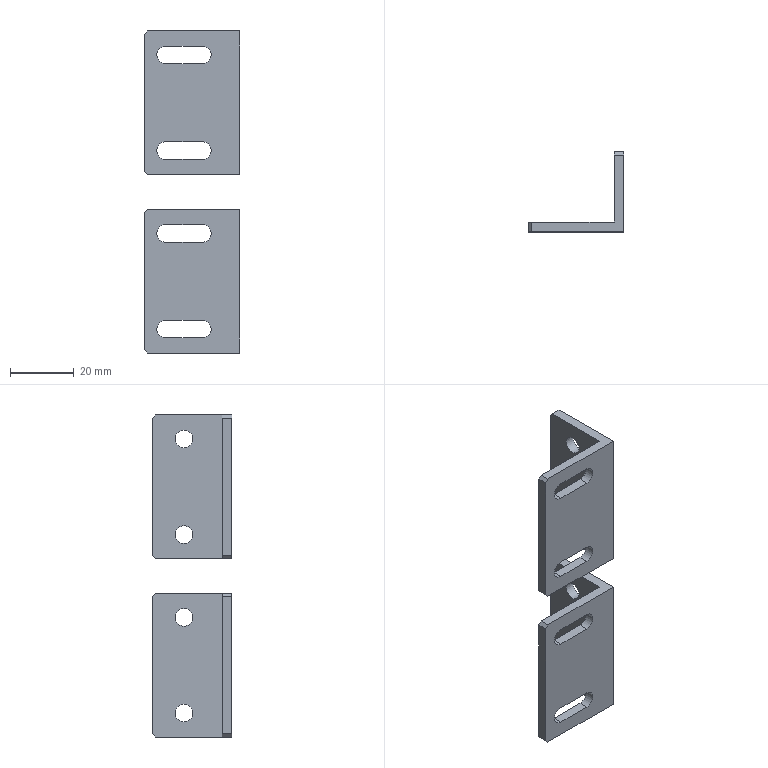Part | 2 solids | 44 faces | box 30 x 25 x 101 mm | volume 12699 mm3 | plane 32 | cylinder 12 | commonest cylinder face diameters 5.5 x12
STEP:
#1=CARTESIAN_POINT('',(-3.,25.,34.5));
#2=VERTEX_POINT('',#1);
#3=CARTESIAN_POINT('',(-3.,24.,33.5));
#4=VERTEX_POINT('',#3);
#5=CARTESIAN_POINT('',(-3.,34.5,44.));
#6=DIRECTION('',(0.,-0.7071,-0.7071));
#7=VECTOR('',#6,1000.);
#8=LINE('',#5,#7);
#9=EDGE_CURVE('',#2,#4,#8,.T.);
#10=ORIENTED_EDGE('',*,*,#9,.F.);
#11=CARTESIAN_POINT('',(0.,25.,34.5));
#12=VERTEX_POINT('',#11);
#13=CARTESIAN_POINT('',(-3.,25.,34.5));
#14=DIRECTION('',(-1.,0.,0.));
#15=VECTOR('',#14,1000.);
#16=LINE('',#13,#15);
#17=EDGE_CURVE('',#12,#2,#16,.T.);
#18=ORIENTED_EDGE('',*,*,#17,.F.);
#19=CARTESIAN_POINT('',(0.,24.,33.5));
#20=VERTEX_POINT('',#19);
#21=CARTESIAN_POINT('',(0.,24.,33.5));
#22=DIRECTION('',(0.,0.7071,0.7071));
#23=VECTOR('',#22,1000.);
#24=LINE('',#21,#23);
#25=EDGE_CURVE('',#20,#12,#24,.T.);
#26=ORIENTED_EDGE('',*,*,#25,.F.);
#27=CARTESIAN_POINT('',(0.,24.,33.5));
#28=DIRECTION('',(1.,0.,0.));
#29=VECTOR('',#28,1000.);
#30=LINE('',#27,#29);
#31=EDGE_CURVE('',#4,#20,#30,.T.);
#32=ORIENTED_EDGE('',*,*,#31,.F.);
#33=EDGE_LOOP('',(#10,#18,#26,#32));
#34=FACE_BOUND('',#33,.T.);
#35=CARTESIAN_POINT('',(0.,24.,33.5));
#36=DIRECTION('',(0.,-0.7071,0.7071));
#37=DIRECTION('',(1.,0.,0.));
#38=AXIS2_PLACEMENT_3D('',#35,#36,#37);
#39=PLANE('',#38);
#40=ADVANCED_FACE('',(#34),#39,.F.);
#41=CARTESIAN_POINT('',(-3.,24.,78.5));
#42=VERTEX_POINT('',#41);
#43=CARTESIAN_POINT('',(-3.,25.,77.5));
#44=VERTEX_POINT('',#43);
#45=CARTESIAN_POINT('',(-3.,12.,90.5));
#46=DIRECTION('',(0.,0.7071,-0.7071));
#47=VECTOR('',#46,1000.);
#48=LINE('',#45,#47);
#49=EDGE_CURVE('',#42,#44,#48,.T.);
#50=ORIENTED_EDGE('',*,*,#49,.F.);
#51=CARTESIAN_POINT('',(0.,24.,78.5));
#52=VERTEX_POINT('',#51);
#53=CARTESIAN_POINT('',(-3.,24.,78.5));
#54=DIRECTION('',(-1.,0.,0.));
#55=VECTOR('',#54,1000.);
#56=LINE('',#53,#55);
#57=EDGE_CURVE('',#52,#42,#56,.T.);
#58=ORIENTED_EDGE('',*,*,#57,.F.);
#59=CARTESIAN_POINT('',(0.,25.,77.5));
#60=VERTEX_POINT('',#59);
#61=CARTESIAN_POINT('',(0.,25.,77.5));
#62=DIRECTION('',(0.,-0.7071,0.7071));
#63=VECTOR('',#62,1000.);
#64=LINE('',#61,#63);
#65=EDGE_CURVE('',#60,#52,#64,.T.);
#66=ORIENTED_EDGE('',*,*,#65,.F.);
#67=CARTESIAN_POINT('',(0.,25.,77.5));
#68=DIRECTION('',(1.,0.,0.));
#69=VECTOR('',#68,1000.);
#70=LINE('',#67,#69);
#71=EDGE_CURVE('',#44,#60,#70,.T.);
#72=ORIENTED_EDGE('',*,*,#71,.F.);
#73=EDGE_LOOP('',(#50,#58,#66,#72));
#74=FACE_BOUND('',#73,.T.);
#75=CARTESIAN_POINT('',(-3.,25.,77.5));
#76=DIRECTION('',(0.,0.7071,0.7071));
#77=DIRECTION('',(-1.,0.,0.));
#78=AXIS2_PLACEMENT_3D('',#75,#76,#77);
#79=PLANE('',#78);
#80=ADVANCED_FACE('',(#74),#79,.T.);
#81=CARTESIAN_POINT('',(-29.,0.,78.5));
#82=VERTEX_POINT('',#81);
#83=CARTESIAN_POINT('',(-30.,0.,77.5));
#84=VERTEX_POINT('',#83);
#85=CARTESIAN_POINT('',(-30.,0.,77.5));
#86=DIRECTION('',(-0.7071,0.,-0.7071));
#87=VECTOR('',#86,1000.);
#88=LINE('',#85,#87);
#89=EDGE_CURVE('',#82,#84,#88,.T.);
#90=ORIENTED_EDGE('',*,*,#89,.F.);
#91=CARTESIAN_POINT('',(-29.,3.,78.5));
#92=VERTEX_POINT('',#91);
#93=CARTESIAN_POINT('',(-29.,0.,78.5));
#94=DIRECTION('',(0.,-1.,0.));
#95=VECTOR('',#94,1000.);
#96=LINE('',#93,#95);
#97=EDGE_CURVE('',#92,#82,#96,.T.);
#98=ORIENTED_EDGE('',*,*,#97,.F.);
#99=CARTESIAN_POINT('',(-30.,3.,77.5));
#100=VERTEX_POINT('',#99);
#101=CARTESIAN_POINT('',(-14.5,3.,93.));
#102=DIRECTION('',(0.7071,0.,0.7071));
#103=VECTOR('',#102,1000.);
#104=LINE('',#101,#103);
#105=EDGE_CURVE('',#100,#92,#104,.T.);
#106=ORIENTED_EDGE('',*,*,#105,.F.);
#107=CARTESIAN_POINT('',(-30.,3.,77.5));
#108=DIRECTION('',(0.,1.,0.));
#109=VECTOR('',#108,1000.);
#110=LINE('',#107,#109);
#111=EDGE_CURVE('',#84,#100,#110,.T.);
#112=ORIENTED_EDGE('',*,*,#111,.F.);
#113=EDGE_LOOP('',(#90,#98,#106,#112));
#114=FACE_BOUND('',#113,.T.);
#115=CARTESIAN_POINT('',(-30.,0.,77.5));
#116=DIRECTION('',(-0.7071,0.,0.7071));
#117=DIRECTION('',(0.,-1.,0.));
#118=AXIS2_PLACEMENT_3D('',#115,#116,#117);
#119=PLANE('',#118);
#120=ADVANCED_FACE('',(#114),#119,.T.);
#121=CARTESIAN_POINT('',(-30.,0.,34.5));
#122=VERTEX_POINT('',#121);
#123=CARTESIAN_POINT('',(-29.,0.,33.5));
#124=VERTEX_POINT('',#123);
#125=CARTESIAN_POINT('',(-29.,0.,33.5));
#126=DIRECTION('',(0.7071,0.,-0.7071));
#127=VECTOR('',#126,1000.);
#128=LINE('',#125,#127);
#129=EDGE_CURVE('',#122,#124,#128,.T.);
#130=ORIENTED_EDGE('',*,*,#129,.F.);
#131=CARTESIAN_POINT('',(-30.,3.,34.5));
#132=VERTEX_POINT('',#131);
#133=CARTESIAN_POINT('',(-30.,0.,34.5));
#134=DIRECTION('',(0.,-1.,0.));
#135=VECTOR('',#134,1000.);
#136=LINE('',#133,#135);
#137=EDGE_CURVE('',#132,#122,#136,.T.);
#138=ORIENTED_EDGE('',*,*,#137,.F.);
#139=CARTESIAN_POINT('',(-29.,3.,33.5));
#140=VERTEX_POINT('',#139);
#141=CARTESIAN_POINT('',(-37.,3.,41.5));
#142=DIRECTION('',(-0.7071,0.,0.7071));
#143=VECTOR('',#142,1000.);
#144=LINE('',#141,#143);
#145=EDGE_CURVE('',#140,#132,#144,.T.);
#146=ORIENTED_EDGE('',*,*,#145,.F.);
#147=CARTESIAN_POINT('',(-29.,0.,33.5));
#148=DIRECTION('',(0.,1.,0.));
#149=VECTOR('',#148,1000.);
#150=LINE('',#147,#149);
#151=EDGE_CURVE('',#124,#140,#150,.T.);
#152=ORIENTED_EDGE('',*,*,#151,.F.);
#153=EDGE_LOOP('',(#130,#138,#146,#152));
#154=FACE_BOUND('',#153,.T.);
#155=CARTESIAN_POINT('',(-29.,0.,33.5));
#156=DIRECTION('',(0.7071,0.,0.7071));
#157=DIRECTION('',(0.,1.,0.));
#158=AXIS2_PLACEMENT_3D('',#155,#156,#157);
#159=PLANE('',#158);
#160=ADVANCED_FACE('',(#154),#159,.F.);
#161=CARTESIAN_POINT('',(-11.75,3.,43.75));
#162=VERTEX_POINT('',#161);
#163=CARTESIAN_POINT('',(-11.75,0.,43.75));
#164=VERTEX_POINT('',#163);
#165=CARTESIAN_POINT('',(-11.75,3.,43.75));
#166=DIRECTION('',(0.,-1.,0.));
#167=VECTOR('',#166,1000.);
#168=LINE('',#165,#167);
#169=EDGE_CURVE('',#162,#164,#168,.T.);
#170=ORIENTED_EDGE('',*,*,#169,.T.);
#171=CARTESIAN_POINT('',(-23.25,0.,43.75));
#172=VERTEX_POINT('',#171);
#173=CARTESIAN_POINT('',(-23.25,0.,43.75));
#174=DIRECTION('',(1.,0.,0.));
#175=VECTOR('',#174,1000.);
#176=LINE('',#173,#175);
#177=EDGE_CURVE('',#172,#164,#176,.T.);
#178=ORIENTED_EDGE('',*,*,#177,.F.);
#179=CARTESIAN_POINT('',(-23.25,3.,43.75));
#180=VERTEX_POINT('',#179);
#181=CARTESIAN_POINT('',(-23.25,3.,43.75));
#182=DIRECTION('',(0.,1.,0.));
#183=VECTOR('',#182,1000.);
#184=LINE('',#181,#183);
#185=EDGE_CURVE('',#172,#180,#184,.T.);
#186=ORIENTED_EDGE('',*,*,#185,.T.);
#187=CARTESIAN_POINT('',(-23.25,3.,43.75));
#188=DIRECTION('',(1.,0.,0.));
#189=VECTOR('',#188,1000.);
#190=LINE('',#187,#189);
#191=EDGE_CURVE('',#180,#162,#190,.T.);
#192=ORIENTED_EDGE('',*,*,#191,.T.);
#193=EDGE_LOOP('',(#170,#178,#186,#192));
#194=FACE_BOUND('',#193,.T.);
#195=CARTESIAN_POINT('',(-23.25,3.,43.75));
#196=DIRECTION('',(0.,0.,1.));
#197=DIRECTION('',(1.,0.,0.));
#198=AXIS2_PLACEMENT_3D('',#195,#196,#197);
#199=PLANE('',#198);
#200=ADVANCED_FACE('',(#194),#199,.F.);
#201=CARTESIAN_POINT('',(-11.75,0.,38.25));
#202=VERTEX_POINT('',#201);
#203=CARTESIAN_POINT('',(-11.75,3.,38.25));
#204=VERTEX_POINT('',#203);
#205=CARTESIAN_POINT('',(-11.75,3.,38.25));
#206=DIRECTION('',(0.,1.,0.));
#207=VECTOR('',#206,1000.);
#208=LINE('',#205,#207);
#209=EDGE_CURVE('',#202,#204,#208,.T.);
#210=ORIENTED_EDGE('',*,*,#209,.T.);
#211=CARTESIAN_POINT('',(-23.25,3.,38.25));
#212=VERTEX_POINT('',#211);
#213=CARTESIAN_POINT('',(-23.25,3.,38.25));
#214=DIRECTION('',(1.,0.,0.));
#215=VECTOR('',#214,1000.);
#216=LINE('',#213,#215);
#217=EDGE_CURVE('',#212,#204,#216,.T.);
#218=ORIENTED_EDGE('',*,*,#217,.F.);
#219=CARTESIAN_POINT('',(-23.25,0.,38.25));
#220=VERTEX_POINT('',#219);
#221=CARTESIAN_POINT('',(-23.25,3.,38.25));
#222=DIRECTION('',(0.,-1.,0.));
#223=VECTOR('',#222,1000.);
#224=LINE('',#221,#223);
#225=EDGE_CURVE('',#212,#220,#224,.T.);
#226=ORIENTED_EDGE('',*,*,#225,.T.);
#227=CARTESIAN_POINT('',(-23.25,0.,38.25));
#228=DIRECTION('',(1.,0.,0.));
#229=VECTOR('',#228,1000.);
#230=LINE('',#227,#229);
#231=EDGE_CURVE('',#220,#202,#230,.T.);
#232=ORIENTED_EDGE('',*,*,#231,.T.);
#233=EDGE_LOOP('',(#210,#218,#226,#232));
#234=FACE_BOUND('',#233,.T.);
#235=CARTESIAN_POINT('',(-23.25,3.,38.25));
#236=DIRECTION('',(0.,0.,-1.));
#237=DIRECTION('',(-1.,0.,0.));
#238=AXIS2_PLACEMENT_3D('',#235,#236,#237);
#239=PLANE('',#238);
#240=ADVANCED_FACE('',(#234),#239,.F.);
#241=CARTESIAN_POINT('',(-23.25,3.,41.));
#242=DIRECTION('',(0.,1.,0.));
#243=DIRECTION('',(0.,0.,1.));
#244=AXIS2_PLACEMENT_3D('',#241,#242,#243);
#245=CIRCLE('',#244,2.75);
#246=EDGE_CURVE('',#212,#180,#245,.T.);
#247=ORIENTED_EDGE('',*,*,#246,.T.);
#248=ORIENTED_EDGE('',*,*,#185,.F.);
#249=CARTESIAN_POINT('',(-23.25,0.,41.));
#250=DIRECTION('',(0.,1.,0.));
#251=DIRECTION('',(0.,0.,1.));
#252=AXIS2_PLACEMENT_3D('',#249,#250,#251);
#253=CIRCLE('',#252,2.75);
#254=EDGE_CURVE('',#220,#172,#253,.T.);
#255=ORIENTED_EDGE('',*,*,#254,.F.);
#256=ORIENTED_EDGE('',*,*,#225,.F.);
#257=EDGE_LOOP('',(#247,#248,#255,#256));
#258=FACE_BOUND('',#257,.T.);
#259=CARTESIAN_POINT('',(-23.25,3.,41.));
#260=DIRECTION('',(0.,1.,0.));
#261=DIRECTION('',(0.,0.,1.));
#262=AXIS2_PLACEMENT_3D('',#259,#260,#261);
#263=CYLINDRICAL_SURFACE('',#262,2.75);
#264=ADVANCED_FACE('',(#258),#263,.F.);
#265=CARTESIAN_POINT('',(-11.75,0.,41.));
#266=DIRECTION('',(0.,1.,0.));
#267=DIRECTION('',(0.,0.,1.));
#268=AXIS2_PLACEMENT_3D('',#265,#266,#267);
#269=CIRCLE('',#268,2.75);
#270=EDGE_CURVE('',#164,#202,#269,.T.);
#271=ORIENTED_EDGE('',*,*,#270,.F.);
#272=ORIENTED_EDGE('',*,*,#169,.F.);
#273=CARTESIAN_POINT('',(-11.75,3.,41.));
#274=DIRECTION('',(0.,1.,0.));
#275=DIRECTION('',(0.,0.,1.));
#276=AXIS2_PLACEMENT_3D('',#273,#274,#275);
#277=CIRCLE('',#276,2.75);
#278=EDGE_CURVE('',#162,#204,#277,.T.);
#279=ORIENTED_EDGE('',*,*,#278,.T.);
#280=ORIENTED_EDGE('',*,*,#209,.F.);
#281=EDGE_LOOP('',(#271,#272,#279,#280));
#282=FACE_BOUND('',#281,.T.);
#283=CARTESIAN_POINT('',(-11.75,3.,41.));
#284=DIRECTION('',(0.,1.,0.));
#285=DIRECTION('',(0.,0.,1.));
#286=AXIS2_PLACEMENT_3D('',#283,#284,#285);
#287=CYLINDRICAL_SURFACE('',#286,2.75);
#288=ADVANCED_FACE('',(#282),#287,.F.);
#289=CARTESIAN_POINT('',(-11.75,3.,73.75));
#290=VERTEX_POINT('',#289);
#291=CARTESIAN_POINT('',(-11.75,0.,73.75));
#292=VERTEX_POINT('',#291);
#293=CARTESIAN_POINT('',(-11.75,3.,73.75));
#294=DIRECTION('',(0.,-1.,0.));
#295=VECTOR('',#294,1000.);
#296=LINE('',#293,#295);
#297=EDGE_CURVE('',#290,#292,#296,.T.);
#298=ORIENTED_EDGE('',*,*,#297,.T.);
#299=CARTESIAN_POINT('',(-23.25,0.,73.75));
#300=VERTEX_POINT('',#299);
#301=CARTESIAN_POINT('',(-23.25,0.,73.75));
#302=DIRECTION('',(1.,0.,0.));
#303=VECTOR('',#302,1000.);
#304=LINE('',#301,#303);
#305=EDGE_CURVE('',#300,#292,#304,.T.);
#306=ORIENTED_EDGE('',*,*,#305,.F.);
#307=CARTESIAN_POINT('',(-23.25,3.,73.75));
#308=VERTEX_POINT('',#307);
#309=CARTESIAN_POINT('',(-23.25,3.,73.75));
#310=DIRECTION('',(0.,1.,0.));
#311=VECTOR('',#310,1000.);
#312=LINE('',#309,#311);
#313=EDGE_CURVE('',#300,#308,#312,.T.);
#314=ORIENTED_EDGE('',*,*,#313,.T.);
#315=CARTESIAN_POINT('',(-23.25,3.,73.75));
#316=DIRECTION('',(1.,0.,0.));
#317=VECTOR('',#316,1000.);
#318=LINE('',#315,#317);
#319=EDGE_CURVE('',#308,#290,#318,.T.);
#320=ORIENTED_EDGE('',*,*,#319,.T.);
#321=EDGE_LOOP('',(#298,#306,#314,#320));
#322=FACE_BOUND('',#321,.T.);
#323=CARTESIAN_POINT('',(-23.25,3.,73.75));
#324=DIRECTION('',(0.,0.,1.));
#325=DIRECTION('',(1.,0.,0.));
#326=AXIS2_PLACEMENT_3D('',#323,#324,#325);
#327=PLANE('',#326);
#328=ADVANCED_FACE('',(#322),#327,.F.);
#329=CARTESIAN_POINT('',(-11.75,0.,68.25));
#330=VERTEX_POINT('',#329);
#331=CARTESIAN_POINT('',(-11.75,3.,68.25));
#332=VERTEX_POINT('',#331);
#333=CARTESIAN_POINT('',(-11.75,3.,68.25));
#334=DIRECTION('',(0.,1.,0.));
#335=VECTOR('',#334,1000.);
#336=LINE('',#333,#335);
#337=EDGE_CURVE('',#330,#332,#336,.T.);
#338=ORIENTED_EDGE('',*,*,#337,.T.);
#339=CARTESIAN_POINT('',(-23.25,3.,68.25));
#340=VERTEX_POINT('',#339);
#341=CARTESIAN_POINT('',(-23.25,3.,68.25));
#342=DIRECTION('',(1.,0.,0.));
#343=VECTOR('',#342,1000.);
#344=LINE('',#341,#343);
#345=EDGE_CURVE('',#340,#332,#344,.T.);
#346=ORIENTED_EDGE('',*,*,#345,.F.);
#347=CARTESIAN_POINT('',(-23.25,0.,68.25));
#348=VERTEX_POINT('',#347);
#349=CARTESIAN_POINT('',(-23.25,3.,68.25));
#350=DIRECTION('',(0.,-1.,0.));
#351=VECTOR('',#350,1000.);
#352=LINE('',#349,#351);
#353=EDGE_CURVE('',#340,#348,#352,.T.);
#354=ORIENTED_EDGE('',*,*,#353,.T.);
#355=CARTESIAN_POINT('',(-23.25,0.,68.25));
#356=DIRECTION('',(1.,0.,0.));
#357=VECTOR('',#356,1000.);
#358=LINE('',#355,#357);
#359=EDGE_CURVE('',#348,#330,#358,.T.);
#360=ORIENTED_EDGE('',*,*,#359,.T.);
#361=EDGE_LOOP('',(#338,#346,#354,#360));
#362=FACE_BOUND('',#361,.T.);
#363=CARTESIAN_POINT('',(-23.25,3.,68.25));
#364=DIRECTION('',(0.,0.,-1.));
#365=DIRECTION('',(-1.,0.,0.));
#366=AXIS2_PLACEMENT_3D('',#363,#364,#365);
#367=PLANE('',#366);
#368=ADVANCED_FACE('',(#362),#367,.F.);
#369=CARTESIAN_POINT('',(-23.25,3.,71.));
#370=DIRECTION('',(0.,1.,0.));
#371=DIRECTION('',(0.,0.,1.));
#372=AXIS2_PLACEMENT_3D('',#369,#370,#371);
#373=CIRCLE('',#372,2.75);
#374=EDGE_CURVE('',#340,#308,#373,.T.);
#375=ORIENTED_EDGE('',*,*,#374,.T.);
#376=ORIENTED_EDGE('',*,*,#313,.F.);
#377=CARTESIAN_POINT('',(-23.25,0.,71.));
#378=DIRECTION('',(0.,1.,0.));
#379=DIRECTION('',(0.,0.,1.));
#380=AXIS2_PLACEMENT_3D('',#377,#378,#379);
#381=CIRCLE('',#380,2.75);
#382=EDGE_CURVE('',#348,#300,#381,.T.);
#383=ORIENTED_EDGE('',*,*,#382,.F.);
#384=ORIENTED_EDGE('',*,*,#353,.F.);
#385=EDGE_LOOP('',(#375,#376,#383,#384));
#386=FACE_BOUND('',#385,.T.);
#387=CARTESIAN_POINT('',(-23.25,3.,71.));
#388=DIRECTION('',(0.,1.,0.));
#389=DIRECTION('',(0.,0.,1.));
#390=AXIS2_PLACEMENT_3D('',#387,#388,#389);
#391=CYLINDRICAL_SURFACE('',#390,2.75);
#392=ADVANCED_FACE('',(#386),#391,.F.);
#393=CARTESIAN_POINT('',(-11.75,0.,71.));
#394=DIRECTION('',(0.,1.,0.));
#395=DIRECTION('',(0.,0.,1.));
#396=AXIS2_PLACEMENT_3D('',#393,#394,#395);
#397=CIRCLE('',#396,2.75);
#398=EDGE_CURVE('',#292,#330,#397,.T.);
#399=ORIENTED_EDGE('',*,*,#398,.F.);
#400=ORIENTED_EDGE('',*,*,#297,.F.);
#401=CARTESIAN_POINT('',(-11.75,3.,71.));
#402=DIRECTION('',(0.,1.,0.));
#403=DIRECTION('',(0.,0.,1.));
#404=AXIS2_PLACEMENT_3D('',#401,#402,#403);
#405=CIRCLE('',#404,2.75);
#406=EDGE_CURVE('',#290,#332,#405,.T.);
#407=ORIENTED_EDGE('',*,*,#406,.T.);
#408=ORIENTED_EDGE('',*,*,#337,.F.);
#409=EDGE_LOOP('',(#399,#400,#407,#408));
#410=FACE_BOUND('',#409,.T.);
#411=CARTESIAN_POINT('',(-11.75,3.,71.));
#412=DIRECTION('',(0.,1.,0.));
#413=DIRECTION('',(0.,0.,1.));
#414=AXIS2_PLACEMENT_3D('',#411,#412,#413);
#415=CYLINDRICAL_SURFACE('',#414,2.75);
#416=ADVANCED_FACE('',(#410),#415,.F.);
#417=CARTESIAN_POINT('',(-3.,15.,43.75));
#418=VERTEX_POINT('',#417);
#419=CARTESIAN_POINT('',(-3.,15.,41.));
#420=DIRECTION('',(-1.,0.,0.));
#421=DIRECTION('',(0.,0.,1.));
#422=AXIS2_PLACEMENT_3D('',#419,#420,#421);
#423=CIRCLE('',#422,2.75);
#424=EDGE_CURVE('',#418,#418,#423,.T.);
#425=ORIENTED_EDGE('',*,*,#424,.T.);
#426=EDGE_LOOP('',(#425));
#427=FACE_BOUND('',#426,.T.);
#428=CARTESIAN_POINT('',(0.,15.,43.75));
#429=VERTEX_POINT('',#428);
#430=CARTESIAN_POINT('',(0.,15.,41.));
#431=DIRECTION('',(-1.,0.,0.));
#432=DIRECTION('',(0.,0.,1.));
#433=AXIS2_PLACEMENT_3D('',#430,#431,#432);
#434=CIRCLE('',#433,2.75);
#435=EDGE_CURVE('',#429,#429,#434,.T.);
#436=ORIENTED_EDGE('',*,*,#435,.F.);
#437=EDGE_LOOP('',(#436));
#438=FACE_BOUND('',#437,.T.);
#439=CARTESIAN_POINT('',(-3.,15.,41.));
#440=DIRECTION('',(-1.,0.,0.));
#441=DIRECTION('',(0.,0.,1.));
#442=AXIS2_PLACEMENT_3D('',#439,#440,#441);
#443=CYLINDRICAL_SURFACE('',#442,2.75);
#444=ADVANCED_FACE('',(#427,#438),#443,.F.);
#445=CARTESIAN_POINT('',(-3.,15.,73.75));
#446=VERTEX_POINT('',#445);
#447=CARTESIAN_POINT('',(-3.,15.,71.));
#448=DIRECTION('',(-1.,0.,0.));
#449=DIRECTION('',(0.,0.,1.));
#450=AXIS2_PLACEMENT_3D('',#447,#448,#449);
#451=CIRCLE('',#450,2.75);
#452=EDGE_CURVE('',#446,#446,#451,.T.);
#453=ORIENTED_EDGE('',*,*,#452,.T.);
#454=EDGE_LOOP('',(#453));
#455=FACE_BOUND('',#454,.T.);
#456=CARTESIAN_POINT('',(0.,15.,73.75));
#457=VERTEX_POINT('',#456);
#458=CARTESIAN_POINT('',(0.,15.,71.));
#459=DIRECTION('',(-1.,0.,0.));
#460=DIRECTION('',(0.,0.,1.));
#461=AXIS2_PLACEMENT_3D('',#458,#459,#460);
#462=CIRCLE('',#461,2.75);
#463=EDGE_CURVE('',#457,#457,#462,.T.);
#464=ORIENTED_EDGE('',*,*,#463,.F.);
#465=EDGE_LOOP('',(#464));
#466=FACE_BOUND('',#465,.T.);
#467=CARTESIAN_POINT('',(-3.,15.,71.));
#468=DIRECTION('',(-1.,0.,0.));
#469=DIRECTION('',(0.,0.,1.));
#470=AXIS2_PLACEMENT_3D('',#467,#468,#469);
#471=CYLINDRICAL_SURFACE('',#470,2.75);
#472=ADVANCED_FACE('',(#455,#466),#471,.F.);
#473=CARTESIAN_POINT('',(0.,0.,33.5));
#474=VERTEX_POINT('',#473);
#475=CARTESIAN_POINT('',(0.,0.,33.5));
#476=DIRECTION('',(1.,0.,0.));
#477=VECTOR('',#476,1000.);
#478=LINE('',#475,#477);
#479=EDGE_CURVE('',#124,#474,#478,.T.);
#480=ORIENTED_EDGE('',*,*,#479,.F.);
#481=ORIENTED_EDGE('',*,*,#151,.T.);
#482=CARTESIAN_POINT('',(-3.,3.,33.5));
#483=VERTEX_POINT('',#482);
#484=CARTESIAN_POINT('',(0.,3.,33.5));
#485=DIRECTION('',(1.,0.,0.));
#486=VECTOR('',#485,1000.);
#487=LINE('',#484,#486);
#488=EDGE_CURVE('',#140,#483,#487,.T.);
#489=ORIENTED_EDGE('',*,*,#488,.T.);
#490=CARTESIAN_POINT('',(-3.,0.,33.5));
#491=DIRECTION('',(0.,1.,0.));
#492=VECTOR('',#491,1000.);
#493=LINE('',#490,#492);
#494=EDGE_CURVE('',#483,#4,#493,.T.);
#495=ORIENTED_EDGE('',*,*,#494,.T.);
#496=ORIENTED_EDGE('',*,*,#31,.T.);
#497=CARTESIAN_POINT('',(0.,0.,33.5));
#498=DIRECTION('',(0.,1.,0.));
#499=VECTOR('',#498,1000.);
#500=LINE('',#497,#499);
#501=EDGE_CURVE('',#474,#20,#500,.T.);
#502=ORIENTED_EDGE('',*,*,#501,.F.);
#503=EDGE_LOOP('',(#480,#481,#489,#495,#496,#502));
#504=FACE_BOUND('',#503,.T.);
#505=CARTESIAN_POINT('',(0.,0.,33.5));
#506=DIRECTION('',(0.,0.,-1.));
#507=DIRECTION('',(-1.,0.,0.));
#508=AXIS2_PLACEMENT_3D('',#505,#506,#507);
#509=PLANE('',#508);
#510=ADVANCED_FACE('',(#504),#509,.T.);
#511=CARTESIAN_POINT('',(-3.,3.,78.5));
#512=VERTEX_POINT('',#511);
#513=CARTESIAN_POINT('',(0.,3.,78.5));
#514=DIRECTION('',(1.,0.,0.));
#515=VECTOR('',#514,1000.);
#516=LINE('',#513,#515);
#517=EDGE_CURVE('',#92,#512,#516,.T.);
#518=ORIENTED_EDGE('',*,*,#517,.F.);
#519=ORIENTED_EDGE('',*,*,#97,.T.);
#520=CARTESIAN_POINT('',(0.,0.,78.5));
#521=VERTEX_POINT('',#520);
#522=CARTESIAN_POINT('',(0.,0.,78.5));
#523=DIRECTION('',(1.,0.,0.));
#524=VECTOR('',#523,1000.);
#525=LINE('',#522,#524);
#526=EDGE_CURVE('',#82,#521,#525,.T.);
#527=ORIENTED_EDGE('',*,*,#526,.T.);
#528=CARTESIAN_POINT('',(0.,0.,78.5));
#529=DIRECTION('',(0.,1.,0.));
#530=VECTOR('',#529,1000.);
#531=LINE('',#528,#530);
#532=EDGE_CURVE('',#521,#52,#531,.T.);
#533=ORIENTED_EDGE('',*,*,#532,.T.);
#534=ORIENTED_EDGE('',*,*,#57,.T.);
#535=CARTESIAN_POINT('',(-3.,0.,78.5));
#536=DIRECTION('',(0.,1.,0.));
#537=VECTOR('',#536,1000.);
#538=LINE('',#535,#537);
#539=EDGE_CURVE('',#512,#42,#538,.T.);
#540=ORIENTED_EDGE('',*,*,#539,.F.);
#541=EDGE_LOOP('',(#518,#519,#527,#533,#534,#540));
#542=FACE_BOUND('',#541,.T.);
#543=CARTESIAN_POINT('',(0.,0.,78.5));
#544=DIRECTION('',(0.,0.,-1.));
#545=DIRECTION('',(-1.,0.,0.));
#546=AXIS2_PLACEMENT_3D('',#543,#544,#545);
#547=PLANE('',#546);
#548=ADVANCED_FACE('',(#542),#547,.F.);
#549=CARTESIAN_POINT('',(-30.,0.,78.5));
#550=DIRECTION('',(0.,0.,-1.));
#551=VECTOR('',#550,1000.);
#552=LINE('',#549,#551);
#553=EDGE_CURVE('',#84,#122,#552,.T.);
#554=ORIENTED_EDGE('',*,*,#553,.T.);
#555=ORIENTED_EDGE('',*,*,#129,.T.);
#556=ORIENTED_EDGE('',*,*,#479,.T.);
#557=CARTESIAN_POINT('',(0.,0.,78.5));
#558=DIRECTION('',(0.,0.,-1.));
#559=VECTOR('',#558,1000.);
#560=LINE('',#557,#559);
#561=EDGE_CURVE('',#521,#474,#560,.T.);
#562=ORIENTED_EDGE('',*,*,#561,.F.);
#563=ORIENTED_EDGE('',*,*,#526,.F.);
#564=ORIENTED_EDGE('',*,*,#89,.T.);
#565=EDGE_LOOP('',(#554,#555,#556,#562,#563,#564));
#566=FACE_BOUND('',#565,.T.);
#567=ORIENTED_EDGE('',*,*,#305,.T.);
#568=ORIENTED_EDGE('',*,*,#398,.T.);
#569=ORIENTED_EDGE('',*,*,#359,.F.);
#570=ORIENTED_EDGE('',*,*,#382,.T.);
#571=EDGE_LOOP('',(#567,#568,#569,#570));
#572=FACE_BOUND('',#571,.T.);
#573=ORIENTED_EDGE('',*,*,#254,.T.);
#574=ORIENTED_EDGE('',*,*,#177,.T.);
#575=ORIENTED_EDGE('',*,*,#270,.T.);
#576=ORIENTED_EDGE('',*,*,#231,.F.);
#577=EDGE_LOOP('',(#573,#574,#575,#576));
#578=FACE_BOUND('',#577,.T.);
#579=CARTESIAN_POINT('',(0.,0.,78.5));
#580=DIRECTION('',(0.,1.,0.));
#581=DIRECTION('',(-1.,0.,0.));
#582=AXIS2_PLACEMENT_3D('',#579,#580,#581);
#583=PLANE('',#582);
#584=ADVANCED_FACE('',(#566,#572,#578),#583,.F.);
#585=CARTESIAN_POINT('',(-30.,3.,78.5));
#586=DIRECTION('',(0.,0.,-1.));
#587=VECTOR('',#586,1000.);
#588=LINE('',#585,#587);
#589=EDGE_CURVE('',#100,#132,#588,.T.);
#590=ORIENTED_EDGE('',*,*,#589,.T.);
#591=ORIENTED_EDGE('',*,*,#137,.T.);
#592=ORIENTED_EDGE('',*,*,#553,.F.);
#593=ORIENTED_EDGE('',*,*,#111,.T.);
#594=EDGE_LOOP('',(#590,#591,#592,#593));
#595=FACE_BOUND('',#594,.T.);
#596=CARTESIAN_POINT('',(-30.,0.,78.5));
#597=DIRECTION('',(-1.,0.,0.));
#598=DIRECTION('',(0.,0.,1.));
#599=AXIS2_PLACEMENT_3D('',#596,#597,#598);
#600=PLANE('',#599);
#601=ADVANCED_FACE('',(#595),#600,.T.);
#602=ORIENTED_EDGE('',*,*,#488,.F.);
#603=ORIENTED_EDGE('',*,*,#145,.T.);
#604=ORIENTED_EDGE('',*,*,#589,.F.);
#605=ORIENTED_EDGE('',*,*,#105,.T.);
#606=ORIENTED_EDGE('',*,*,#517,.T.);
#607=CARTESIAN_POINT('',(-3.,3.,78.5));
#608=DIRECTION('',(0.,0.,-1.));
#609=VECTOR('',#608,1000.);
#610=LINE('',#607,#609);
#611=EDGE_CURVE('',#512,#483,#610,.T.);
#612=ORIENTED_EDGE('',*,*,#611,.T.);
#613=EDGE_LOOP('',(#602,#603,#604,#605,#606,#612));
#614=FACE_BOUND('',#613,.T.);
#615=ORIENTED_EDGE('',*,*,#319,.F.);
#616=ORIENTED_EDGE('',*,*,#374,.F.);
#617=ORIENTED_EDGE('',*,*,#345,.T.);
#618=ORIENTED_EDGE('',*,*,#406,.F.);
#619=EDGE_LOOP('',(#615,#616,#617,#618));
#620=FACE_BOUND('',#619,.T.);
#621=ORIENTED_EDGE('',*,*,#246,.F.);
#622=ORIENTED_EDGE('',*,*,#217,.T.);
#623=ORIENTED_EDGE('',*,*,#278,.F.);
#624=ORIENTED_EDGE('',*,*,#191,.F.);
#625=EDGE_LOOP('',(#621,#622,#623,#624));
#626=FACE_BOUND('',#625,.T.);
#627=CARTESIAN_POINT('',(0.,3.,78.5));
#628=DIRECTION('',(0.,1.,0.));
#629=DIRECTION('',(-1.,0.,0.));
#630=AXIS2_PLACEMENT_3D('',#627,#628,#629);
#631=PLANE('',#630);
#632=ADVANCED_FACE('',(#614,#620,#626),#631,.T.);
#633=ORIENTED_EDGE('',*,*,#539,.T.);
#634=ORIENTED_EDGE('',*,*,#49,.T.);
#635=CARTESIAN_POINT('',(-3.,25.,78.5));
#636=DIRECTION('',(0.,0.,-1.));
#637=VECTOR('',#636,1000.);
#638=LINE('',#635,#637);
#639=EDGE_CURVE('',#44,#2,#638,.T.);
#640=ORIENTED_EDGE('',*,*,#639,.T.);
#641=ORIENTED_EDGE('',*,*,#9,.T.);
#642=ORIENTED_EDGE('',*,*,#494,.F.);
#643=ORIENTED_EDGE('',*,*,#611,.F.);
#644=EDGE_LOOP('',(#633,#634,#640,#641,#642,#643));
#645=FACE_BOUND('',#644,.T.);
#646=ORIENTED_EDGE('',*,*,#452,.F.);
#647=EDGE_LOOP('',(#646));
#648=FACE_BOUND('',#647,.T.);
#649=ORIENTED_EDGE('',*,*,#424,.F.);
#650=EDGE_LOOP('',(#649));
#651=FACE_BOUND('',#650,.T.);
#652=CARTESIAN_POINT('',(-3.,0.,78.5));
#653=DIRECTION('',(-1.,0.,0.));
#654=DIRECTION('',(0.,0.,1.));
#655=AXIS2_PLACEMENT_3D('',#652,#653,#654);
#656=PLANE('',#655);
#657=ADVANCED_FACE('',(#645,#648,#651),#656,.T.);
#658=ORIENTED_EDGE('',*,*,#639,.F.);
#659=ORIENTED_EDGE('',*,*,#71,.T.);
#660=CARTESIAN_POINT('',(0.,25.,78.5));
#661=DIRECTION('',(0.,0.,-1.));
#662=VECTOR('',#661,1000.);
#663=LINE('',#660,#662);
#664=EDGE_CURVE('',#60,#12,#663,.T.);
#665=ORIENTED_EDGE('',*,*,#664,.T.);
#666=ORIENTED_EDGE('',*,*,#17,.T.);
#667=EDGE_LOOP('',(#658,#659,#665,#666));
#668=FACE_BOUND('',#667,.T.);
#669=CARTESIAN_POINT('',(-3.,25.,78.5));
#670=DIRECTION('',(0.,1.,0.));
#671=DIRECTION('',(0.,0.,1.));
#672=AXIS2_PLACEMENT_3D('',#669,#670,#671);
#673=PLANE('',#672);
#674=ADVANCED_FACE('',(#668),#673,.T.);
#675=ORIENTED_EDGE('',*,*,#664,.F.);
#676=ORIENTED_EDGE('',*,*,#65,.T.);
#677=ORIENTED_EDGE('',*,*,#532,.F.);
#678=ORIENTED_EDGE('',*,*,#561,.T.);
#679=ORIENTED_EDGE('',*,*,#501,.T.);
#680=ORIENTED_EDGE('',*,*,#25,.T.);
#681=EDGE_LOOP('',(#675,#676,#677,#678,#679,#680));
#682=FACE_BOUND('',#681,.T.);
#683=ORIENTED_EDGE('',*,*,#463,.T.);
#684=EDGE_LOOP('',(#683));
#685=FACE_BOUND('',#684,.T.);
#686=ORIENTED_EDGE('',*,*,#435,.T.);
#687=EDGE_LOOP('',(#686));
#688=FACE_BOUND('',#687,.T.);
#689=CARTESIAN_POINT('',(0.,0.,78.5));
#690=DIRECTION('',(-1.,0.,0.));
#691=DIRECTION('',(0.,0.,1.));
#692=AXIS2_PLACEMENT_3D('',#689,#690,#691);
#693=PLANE('',#692);
#694=ADVANCED_FACE('',(#682,#685,#688),#693,.F.);
#695=CLOSED_SHELL('',(#40,#80,#120,#160,#200,#240,#264,#288,#328,#368,#392,#416,#444,#472,#510,#548,#584,#601,#632,#657,#674,#694));
#696=MANIFOLD_SOLID_BREP('',#695);
#697=CARTESIAN_POINT('',(-3.,25.,-21.5));
#698=VERTEX_POINT('',#697);
#699=CARTESIAN_POINT('',(-3.,24.,-22.5));
#700=VERTEX_POINT('',#699);
#701=CARTESIAN_POINT('',(-3.,34.5,-12.));
#702=DIRECTION('',(0.,-0.7071,-0.7071));
#703=VECTOR('',#702,1000.);
#704=LINE('',#701,#703);
#705=EDGE_CURVE('',#698,#700,#704,.T.);
#706=ORIENTED_EDGE('',*,*,#705,.F.);
#707=CARTESIAN_POINT('',(0.,25.,-21.5));
#708=VERTEX_POINT('',#707);
#709=CARTESIAN_POINT('',(-3.,25.,-21.5));
#710=DIRECTION('',(-1.,0.,0.));
#711=VECTOR('',#710,1000.);
#712=LINE('',#709,#711);
#713=EDGE_CURVE('',#708,#698,#712,.T.);
#714=ORIENTED_EDGE('',*,*,#713,.F.);
#715=CARTESIAN_POINT('',(0.,24.,-22.5));
#716=VERTEX_POINT('',#715);
#717=CARTESIAN_POINT('',(0.,24.,-22.5));
#718=DIRECTION('',(0.,0.7071,0.7071));
#719=VECTOR('',#718,1000.);
#720=LINE('',#717,#719);
#721=EDGE_CURVE('',#716,#708,#720,.T.);
#722=ORIENTED_EDGE('',*,*,#721,.F.);
#723=CARTESIAN_POINT('',(0.,24.,-22.5));
#724=DIRECTION('',(1.,0.,0.));
#725=VECTOR('',#724,1000.);
#726=LINE('',#723,#725);
#727=EDGE_CURVE('',#700,#716,#726,.T.);
#728=ORIENTED_EDGE('',*,*,#727,.F.);
#729=EDGE_LOOP('',(#706,#714,#722,#728));
#730=FACE_BOUND('',#729,.T.);
#731=CARTESIAN_POINT('',(0.,24.,-22.5));
#732=DIRECTION('',(0.,-0.7071,0.7071));
#733=DIRECTION('',(1.,0.,0.));
#734=AXIS2_PLACEMENT_3D('',#731,#732,#733);
#735=PLANE('',#734);
#736=ADVANCED_FACE('',(#730),#735,.F.);
#737=CARTESIAN_POINT('',(-3.,24.,22.5));
#738=VERTEX_POINT('',#737);
#739=CARTESIAN_POINT('',(-3.,25.,21.5));
#740=VERTEX_POINT('',#739);
#741=CARTESIAN_POINT('',(-3.,12.,34.5));
#742=DIRECTION('',(0.,0.7071,-0.7071));
#743=VECTOR('',#742,1000.);
#744=LINE('',#741,#743);
#745=EDGE_CURVE('',#738,#740,#744,.T.);
#746=ORIENTED_EDGE('',*,*,#745,.F.);
#747=CARTESIAN_POINT('',(0.,24.,22.5));
#748=VERTEX_POINT('',#747);
#749=CARTESIAN_POINT('',(-3.,24.,22.5));
#750=DIRECTION('',(-1.,0.,0.));
#751=VECTOR('',#750,1000.);
#752=LINE('',#749,#751);
#753=EDGE_CURVE('',#748,#738,#752,.T.);
#754=ORIENTED_EDGE('',*,*,#753,.F.);
#755=CARTESIAN_POINT('',(0.,25.,21.5));
#756=VERTEX_POINT('',#755);
#757=CARTESIAN_POINT('',(0.,25.,21.5));
#758=DIRECTION('',(0.,-0.7071,0.7071));
#759=VECTOR('',#758,1000.);
#760=LINE('',#757,#759);
#761=EDGE_CURVE('',#756,#748,#760,.T.);
#762=ORIENTED_EDGE('',*,*,#761,.F.);
#763=CARTESIAN_POINT('',(0.,25.,21.5));
#764=DIRECTION('',(1.,0.,0.));
#765=VECTOR('',#764,1000.);
#766=LINE('',#763,#765);
#767=EDGE_CURVE('',#740,#756,#766,.T.);
#768=ORIENTED_EDGE('',*,*,#767,.F.);
#769=EDGE_LOOP('',(#746,#754,#762,#768));
#770=FACE_BOUND('',#769,.T.);
#771=CARTESIAN_POINT('',(-3.,25.,21.5));
#772=DIRECTION('',(0.,0.7071,0.7071));
#773=DIRECTION('',(-1.,0.,0.));
#774=AXIS2_PLACEMENT_3D('',#771,#772,#773);
#775=PLANE('',#774);
#776=ADVANCED_FACE('',(#770),#775,.T.);
#777=CARTESIAN_POINT('',(-29.,0.,22.5));
#778=VERTEX_POINT('',#777);
#779=CARTESIAN_POINT('',(-30.,0.,21.5));
#780=VERTEX_POINT('',#779);
#781=CARTESIAN_POINT('',(-30.,0.,21.5));
#782=DIRECTION('',(-0.7071,0.,-0.7071));
#783=VECTOR('',#782,1000.);
#784=LINE('',#781,#783);
#785=EDGE_CURVE('',#778,#780,#784,.T.);
#786=ORIENTED_EDGE('',*,*,#785,.F.);
#787=CARTESIAN_POINT('',(-29.,3.,22.5));
#788=VERTEX_POINT('',#787);
#789=CARTESIAN_POINT('',(-29.,0.,22.5));
#790=DIRECTION('',(0.,-1.,0.));
#791=VECTOR('',#790,1000.);
#792=LINE('',#789,#791);
#793=EDGE_CURVE('',#788,#778,#792,.T.);
#794=ORIENTED_EDGE('',*,*,#793,.F.);
#795=CARTESIAN_POINT('',(-30.,3.,21.5));
#796=VERTEX_POINT('',#795);
#797=CARTESIAN_POINT('',(-14.5,3.,37.));
#798=DIRECTION('',(0.7071,0.,0.7071));
#799=VECTOR('',#798,1000.);
#800=LINE('',#797,#799);
#801=EDGE_CURVE('',#796,#788,#800,.T.);
#802=ORIENTED_EDGE('',*,*,#801,.F.);
#803=CARTESIAN_POINT('',(-30.,3.,21.5));
#804=DIRECTION('',(0.,1.,0.));
#805=VECTOR('',#804,1000.);
#806=LINE('',#803,#805);
#807=EDGE_CURVE('',#780,#796,#806,.T.);
#808=ORIENTED_EDGE('',*,*,#807,.F.);
#809=EDGE_LOOP('',(#786,#794,#802,#808));
#810=FACE_BOUND('',#809,.T.);
#811=CARTESIAN_POINT('',(-30.,0.,21.5));
#812=DIRECTION('',(-0.7071,0.,0.7071));
#813=DIRECTION('',(0.,-1.,0.));
#814=AXIS2_PLACEMENT_3D('',#811,#812,#813);
#815=PLANE('',#814);
#816=ADVANCED_FACE('',(#810),#815,.T.);
#817=CARTESIAN_POINT('',(-30.,0.,-21.5));
#818=VERTEX_POINT('',#817);
#819=CARTESIAN_POINT('',(-29.,0.,-22.5));
#820=VERTEX_POINT('',#819);
#821=CARTESIAN_POINT('',(-29.,0.,-22.5));
#822=DIRECTION('',(0.7071,0.,-0.7071));
#823=VECTOR('',#822,1000.);
#824=LINE('',#821,#823);
#825=EDGE_CURVE('',#818,#820,#824,.T.);
#826=ORIENTED_EDGE('',*,*,#825,.F.);
#827=CARTESIAN_POINT('',(-30.,3.,-21.5));
#828=VERTEX_POINT('',#827);
#829=CARTESIAN_POINT('',(-30.,0.,-21.5));
#830=DIRECTION('',(0.,-1.,0.));
#831=VECTOR('',#830,1000.);
#832=LINE('',#829,#831);
#833=EDGE_CURVE('',#828,#818,#832,.T.);
#834=ORIENTED_EDGE('',*,*,#833,.F.);
#835=CARTESIAN_POINT('',(-29.,3.,-22.5));
#836=VERTEX_POINT('',#835);
#837=CARTESIAN_POINT('',(-37.,3.,-14.5));
#838=DIRECTION('',(-0.7071,0.,0.7071));
#839=VECTOR('',#838,1000.);
#840=LINE('',#837,#839);
#841=EDGE_CURVE('',#836,#828,#840,.T.);
#842=ORIENTED_EDGE('',*,*,#841,.F.);
#843=CARTESIAN_POINT('',(-29.,0.,-22.5));
#844=DIRECTION('',(0.,1.,0.));
#845=VECTOR('',#844,1000.);
#846=LINE('',#843,#845);
#847=EDGE_CURVE('',#820,#836,#846,.T.);
#848=ORIENTED_EDGE('',*,*,#847,.F.);
#849=EDGE_LOOP('',(#826,#834,#842,#848));
#850=FACE_BOUND('',#849,.T.);
#851=CARTESIAN_POINT('',(-29.,0.,-22.5));
#852=DIRECTION('',(0.7071,0.,0.7071));
#853=DIRECTION('',(0.,1.,0.));
#854=AXIS2_PLACEMENT_3D('',#851,#852,#853);
#855=PLANE('',#854);
#856=ADVANCED_FACE('',(#850),#855,.F.);
#857=CARTESIAN_POINT('',(-11.75,3.,-12.25));
#858=VERTEX_POINT('',#857);
#859=CARTESIAN_POINT('',(-11.75,0.,-12.25));
#860=VERTEX_POINT('',#859);
#861=CARTESIAN_POINT('',(-11.75,3.,-12.25));
#862=DIRECTION('',(0.,-1.,0.));
#863=VECTOR('',#862,1000.);
#864=LINE('',#861,#863);
#865=EDGE_CURVE('',#858,#860,#864,.T.);
#866=ORIENTED_EDGE('',*,*,#865,.T.);
#867=CARTESIAN_POINT('',(-23.25,0.,-12.25));
#868=VERTEX_POINT('',#867);
#869=CARTESIAN_POINT('',(-23.25,0.,-12.25));
#870=DIRECTION('',(1.,0.,0.));
#871=VECTOR('',#870,1000.);
#872=LINE('',#869,#871);
#873=EDGE_CURVE('',#868,#860,#872,.T.);
#874=ORIENTED_EDGE('',*,*,#873,.F.);
#875=CARTESIAN_POINT('',(-23.25,3.,-12.25));
#876=VERTEX_POINT('',#875);
#877=CARTESIAN_POINT('',(-23.25,3.,-12.25));
#878=DIRECTION('',(0.,1.,0.));
#879=VECTOR('',#878,1000.);
#880=LINE('',#877,#879);
#881=EDGE_CURVE('',#868,#876,#880,.T.);
#882=ORIENTED_EDGE('',*,*,#881,.T.);
#883=CARTESIAN_POINT('',(-23.25,3.,-12.25));
#884=DIRECTION('',(1.,0.,0.));
#885=VECTOR('',#884,1000.);
#886=LINE('',#883,#885);
#887=EDGE_CURVE('',#876,#858,#886,.T.);
#888=ORIENTED_EDGE('',*,*,#887,.T.);
#889=EDGE_LOOP('',(#866,#874,#882,#888));
#890=FACE_BOUND('',#889,.T.);
#891=CARTESIAN_POINT('',(-23.25,3.,-12.25));
#892=DIRECTION('',(0.,0.,1.));
#893=DIRECTION('',(1.,0.,0.));
#894=AXIS2_PLACEMENT_3D('',#891,#892,#893);
#895=PLANE('',#894);
#896=ADVANCED_FACE('',(#890),#895,.F.);
#897=CARTESIAN_POINT('',(-11.75,0.,-17.75));
#898=VERTEX_POINT('',#897);
#899=CARTESIAN_POINT('',(-11.75,3.,-17.75));
#900=VERTEX_POINT('',#899);
#901=CARTESIAN_POINT('',(-11.75,3.,-17.75));
#902=DIRECTION('',(0.,1.,0.));
#903=VECTOR('',#902,1000.);
#904=LINE('',#901,#903);
#905=EDGE_CURVE('',#898,#900,#904,.T.);
#906=ORIENTED_EDGE('',*,*,#905,.T.);
#907=CARTESIAN_POINT('',(-23.25,3.,-17.75));
#908=VERTEX_POINT('',#907);
#909=CARTESIAN_POINT('',(-23.25,3.,-17.75));
#910=DIRECTION('',(1.,0.,0.));
#911=VECTOR('',#910,1000.);
#912=LINE('',#909,#911);
#913=EDGE_CURVE('',#908,#900,#912,.T.);
#914=ORIENTED_EDGE('',*,*,#913,.F.);
#915=CARTESIAN_POINT('',(-23.25,0.,-17.75));
#916=VERTEX_POINT('',#915);
#917=CARTESIAN_POINT('',(-23.25,3.,-17.75));
#918=DIRECTION('',(0.,-1.,0.));
#919=VECTOR('',#918,1000.);
#920=LINE('',#917,#919);
#921=EDGE_CURVE('',#908,#916,#920,.T.);
#922=ORIENTED_EDGE('',*,*,#921,.T.);
#923=CARTESIAN_POINT('',(-23.25,0.,-17.75));
#924=DIRECTION('',(1.,0.,0.));
#925=VECTOR('',#924,1000.);
#926=LINE('',#923,#925);
#927=EDGE_CURVE('',#916,#898,#926,.T.);
#928=ORIENTED_EDGE('',*,*,#927,.T.);
#929=EDGE_LOOP('',(#906,#914,#922,#928));
#930=FACE_BOUND('',#929,.T.);
#931=CARTESIAN_POINT('',(-23.25,3.,-17.75));
#932=DIRECTION('',(0.,0.,-1.));
#933=DIRECTION('',(-1.,0.,0.));
#934=AXIS2_PLACEMENT_3D('',#931,#932,#933);
#935=PLANE('',#934);
#936=ADVANCED_FACE('',(#930),#935,.F.);
#937=CARTESIAN_POINT('',(-23.25,3.,-15.));
#938=DIRECTION('',(0.,1.,0.));
#939=DIRECTION('',(0.,0.,1.));
#940=AXIS2_PLACEMENT_3D('',#937,#938,#939);
#941=CIRCLE('',#940,2.75);
#942=EDGE_CURVE('',#908,#876,#941,.T.);
#943=ORIENTED_EDGE('',*,*,#942,.T.);
#944=ORIENTED_EDGE('',*,*,#881,.F.);
#945=CARTESIAN_POINT('',(-23.25,0.,-15.));
#946=DIRECTION('',(0.,1.,0.));
#947=DIRECTION('',(0.,0.,1.));
#948=AXIS2_PLACEMENT_3D('',#945,#946,#947);
#949=CIRCLE('',#948,2.75);
#950=EDGE_CURVE('',#916,#868,#949,.T.);
#951=ORIENTED_EDGE('',*,*,#950,.F.);
#952=ORIENTED_EDGE('',*,*,#921,.F.);
#953=EDGE_LOOP('',(#943,#944,#951,#952));
#954=FACE_BOUND('',#953,.T.);
#955=CARTESIAN_POINT('',(-23.25,3.,-15.));
#956=DIRECTION('',(0.,1.,0.));
#957=DIRECTION('',(0.,0.,1.));
#958=AXIS2_PLACEMENT_3D('',#955,#956,#957);
#959=CYLINDRICAL_SURFACE('',#958,2.75);
#960=ADVANCED_FACE('',(#954),#959,.F.);
#961=CARTESIAN_POINT('',(-11.75,0.,-15.));
#962=DIRECTION('',(0.,1.,0.));
#963=DIRECTION('',(0.,0.,1.));
#964=AXIS2_PLACEMENT_3D('',#961,#962,#963);
#965=CIRCLE('',#964,2.75);
#966=EDGE_CURVE('',#860,#898,#965,.T.);
#967=ORIENTED_EDGE('',*,*,#966,.F.);
#968=ORIENTED_EDGE('',*,*,#865,.F.);
#969=CARTESIAN_POINT('',(-11.75,3.,-15.));
#970=DIRECTION('',(0.,1.,0.));
#971=DIRECTION('',(0.,0.,1.));
#972=AXIS2_PLACEMENT_3D('',#969,#970,#971);
#973=CIRCLE('',#972,2.75);
#974=EDGE_CURVE('',#858,#900,#973,.T.);
#975=ORIENTED_EDGE('',*,*,#974,.T.);
#976=ORIENTED_EDGE('',*,*,#905,.F.);
#977=EDGE_LOOP('',(#967,#968,#975,#976));
#978=FACE_BOUND('',#977,.T.);
#979=CARTESIAN_POINT('',(-11.75,3.,-15.));
#980=DIRECTION('',(0.,1.,0.));
#981=DIRECTION('',(0.,0.,1.));
#982=AXIS2_PLACEMENT_3D('',#979,#980,#981);
#983=CYLINDRICAL_SURFACE('',#982,2.75);
#984=ADVANCED_FACE('',(#978),#983,.F.);
#985=CARTESIAN_POINT('',(-11.75,3.,17.75));
#986=VERTEX_POINT('',#985);
#987=CARTESIAN_POINT('',(-11.75,0.,17.75));
#988=VERTEX_POINT('',#987);
#989=CARTESIAN_POINT('',(-11.75,3.,17.75));
#990=DIRECTION('',(0.,-1.,0.));
#991=VECTOR('',#990,1000.);
#992=LINE('',#989,#991);
#993=EDGE_CURVE('',#986,#988,#992,.T.);
#994=ORIENTED_EDGE('',*,*,#993,.T.);
#995=CARTESIAN_POINT('',(-23.25,0.,17.75));
#996=VERTEX_POINT('',#995);
#997=CARTESIAN_POINT('',(-23.25,0.,17.75));
#998=DIRECTION('',(1.,0.,0.));
#999=VECTOR('',#998,1000.);
#1000=LINE('',#997,#999);
#1001=EDGE_CURVE('',#996,#988,#1000,.T.);
#1002=ORIENTED_EDGE('',*,*,#1001,.F.);
#1003=CARTESIAN_POINT('',(-23.25,3.,17.75));
#1004=VERTEX_POINT('',#1003);
#1005=CARTESIAN_POINT('',(-23.25,3.,17.75));
#1006=DIRECTION('',(0.,1.,0.));
#1007=VECTOR('',#1006,1000.);
#1008=LINE('',#1005,#1007);
#1009=EDGE_CURVE('',#996,#1004,#1008,.T.);
#1010=ORIENTED_EDGE('',*,*,#1009,.T.);
#1011=CARTESIAN_POINT('',(-23.25,3.,17.75));
#1012=DIRECTION('',(1.,0.,0.));
#1013=VECTOR('',#1012,1000.);
#1014=LINE('',#1011,#1013);
#1015=EDGE_CURVE('',#1004,#986,#1014,.T.);
#1016=ORIENTED_EDGE('',*,*,#1015,.T.);
#1017=EDGE_LOOP('',(#994,#1002,#1010,#1016));
#1018=FACE_BOUND('',#1017,.T.);
#1019=CARTESIAN_POINT('',(-23.25,3.,17.75));
#1020=DIRECTION('',(0.,0.,1.));
#1021=DIRECTION('',(1.,0.,0.));
#1022=AXIS2_PLACEMENT_3D('',#1019,#1020,#1021);
#1023=PLANE('',#1022);
#1024=ADVANCED_FACE('',(#1018),#1023,.F.);
#1025=CARTESIAN_POINT('',(-11.75,0.,12.25));
#1026=VERTEX_POINT('',#1025);
#1027=CARTESIAN_POINT('',(-11.75,3.,12.25));
#1028=VERTEX_POINT('',#1027);
#1029=CARTESIAN_POINT('',(-11.75,3.,12.25));
#1030=DIRECTION('',(0.,1.,0.));
#1031=VECTOR('',#1030,1000.);
#1032=LINE('',#1029,#1031);
#1033=EDGE_CURVE('',#1026,#1028,#1032,.T.);
#1034=ORIENTED_EDGE('',*,*,#1033,.T.);
#1035=CARTESIAN_POINT('',(-23.25,3.,12.25));
#1036=VERTEX_POINT('',#1035);
#1037=CARTESIAN_POINT('',(-23.25,3.,12.25));
#1038=DIRECTION('',(1.,0.,0.));
#1039=VECTOR('',#1038,1000.);
#1040=LINE('',#1037,#1039);
#1041=EDGE_CURVE('',#1036,#1028,#1040,.T.);
#1042=ORIENTED_EDGE('',*,*,#1041,.F.);
#1043=CARTESIAN_POINT('',(-23.25,0.,12.25));
#1044=VERTEX_POINT('',#1043);
#1045=CARTESIAN_POINT('',(-23.25,3.,12.25));
#1046=DIRECTION('',(0.,-1.,0.));
#1047=VECTOR('',#1046,1000.);
#1048=LINE('',#1045,#1047);
#1049=EDGE_CURVE('',#1036,#1044,#1048,.T.);
#1050=ORIENTED_EDGE('',*,*,#1049,.T.);
#1051=CARTESIAN_POINT('',(-23.25,0.,12.25));
#1052=DIRECTION('',(1.,0.,0.));
#1053=VECTOR('',#1052,1000.);
#1054=LINE('',#1051,#1053);
#1055=EDGE_CURVE('',#1044,#1026,#1054,.T.);
#1056=ORIENTED_EDGE('',*,*,#1055,.T.);
#1057=EDGE_LOOP('',(#1034,#1042,#1050,#1056));
#1058=FACE_BOUND('',#1057,.T.);
#1059=CARTESIAN_POINT('',(-23.25,3.,12.25));
#1060=DIRECTION('',(0.,0.,-1.));
#1061=DIRECTION('',(-1.,0.,0.));
#1062=AXIS2_PLACEMENT_3D('',#1059,#1060,#1061);
#1063=PLANE('',#1062);
#1064=ADVANCED_FACE('',(#1058),#1063,.F.);
#1065=CARTESIAN_POINT('',(-23.25,3.,15.));
#1066=DIRECTION('',(0.,1.,0.));
#1067=DIRECTION('',(0.,0.,1.));
#1068=AXIS2_PLACEMENT_3D('',#1065,#1066,#1067);
#1069=CIRCLE('',#1068,2.75);
#1070=EDGE_CURVE('',#1036,#1004,#1069,.T.);
#1071=ORIENTED_EDGE('',*,*,#1070,.T.);
#1072=ORIENTED_EDGE('',*,*,#1009,.F.);
#1073=CARTESIAN_POINT('',(-23.25,0.,15.));
#1074=DIRECTION('',(0.,1.,0.));
#1075=DIRECTION('',(0.,0.,1.));
#1076=AXIS2_PLACEMENT_3D('',#1073,#1074,#1075);
#1077=CIRCLE('',#1076,2.75);
#1078=EDGE_CURVE('',#1044,#996,#1077,.T.);
#1079=ORIENTED_EDGE('',*,*,#1078,.F.);
#1080=ORIENTED_EDGE('',*,*,#1049,.F.);
#1081=EDGE_LOOP('',(#1071,#1072,#1079,#1080));
#1082=FACE_BOUND('',#1081,.T.);
#1083=CARTESIAN_POINT('',(-23.25,3.,15.));
#1084=DIRECTION('',(0.,1.,0.));
#1085=DIRECTION('',(0.,0.,1.));
#1086=AXIS2_PLACEMENT_3D('',#1083,#1084,#1085);
#1087=CYLINDRICAL_SURFACE('',#1086,2.75);
#1088=ADVANCED_FACE('',(#1082),#1087,.F.);
#1089=CARTESIAN_POINT('',(-11.75,0.,15.));
#1090=DIRECTION('',(0.,1.,0.));
#1091=DIRECTION('',(0.,0.,1.));
#1092=AXIS2_PLACEMENT_3D('',#1089,#1090,#1091);
#1093=CIRCLE('',#1092,2.75);
#1094=EDGE_CURVE('',#988,#1026,#1093,.T.);
#1095=ORIENTED_EDGE('',*,*,#1094,.F.);
#1096=ORIENTED_EDGE('',*,*,#993,.F.);
#1097=CARTESIAN_POINT('',(-11.75,3.,15.));
#1098=DIRECTION('',(0.,1.,0.));
#1099=DIRECTION('',(0.,0.,1.));
#1100=AXIS2_PLACEMENT_3D('',#1097,#1098,#1099);
#1101=CIRCLE('',#1100,2.75);
#1102=EDGE_CURVE('',#986,#1028,#1101,.T.);
#1103=ORIENTED_EDGE('',*,*,#1102,.T.);
#1104=ORIENTED_EDGE('',*,*,#1033,.F.);
#1105=EDGE_LOOP('',(#1095,#1096,#1103,#1104));
#1106=FACE_BOUND('',#1105,.T.);
#1107=CARTESIAN_POINT('',(-11.75,3.,15.));
#1108=DIRECTION('',(0.,1.,0.));
#1109=DIRECTION('',(0.,0.,1.));
#1110=AXIS2_PLACEMENT_3D('',#1107,#1108,#1109);
#1111=CYLINDRICAL_SURFACE('',#1110,2.75);
#1112=ADVANCED_FACE('',(#1106),#1111,.F.);
#1113=CARTESIAN_POINT('',(-3.,15.,-12.25));
#1114=VERTEX_POINT('',#1113);
#1115=CARTESIAN_POINT('',(-3.,15.,-15.));
#1116=DIRECTION('',(-1.,0.,0.));
#1117=DIRECTION('',(0.,0.,1.));
#1118=AXIS2_PLACEMENT_3D('',#1115,#1116,#1117);
#1119=CIRCLE('',#1118,2.75);
#1120=EDGE_CURVE('',#1114,#1114,#1119,.T.);
#1121=ORIENTED_EDGE('',*,*,#1120,.T.);
#1122=EDGE_LOOP('',(#1121));
#1123=FACE_BOUND('',#1122,.T.);
#1124=CARTESIAN_POINT('',(0.,15.,-12.25));
#1125=VERTEX_POINT('',#1124);
#1126=CARTESIAN_POINT('',(0.,15.,-15.));
#1127=DIRECTION('',(-1.,0.,0.));
#1128=DIRECTION('',(0.,0.,1.));
#1129=AXIS2_PLACEMENT_3D('',#1126,#1127,#1128);
#1130=CIRCLE('',#1129,2.75);
#1131=EDGE_CURVE('',#1125,#1125,#1130,.T.);
#1132=ORIENTED_EDGE('',*,*,#1131,.F.);
#1133=EDGE_LOOP('',(#1132));
#1134=FACE_BOUND('',#1133,.T.);
#1135=CARTESIAN_POINT('',(-3.,15.,-15.));
#1136=DIRECTION('',(-1.,0.,0.));
#1137=DIRECTION('',(0.,0.,1.));
#1138=AXIS2_PLACEMENT_3D('',#1135,#1136,#1137);
#1139=CYLINDRICAL_SURFACE('',#1138,2.75);
#1140=ADVANCED_FACE('',(#1123,#1134),#1139,.F.);
#1141=CARTESIAN_POINT('',(-3.,15.,17.75));
#1142=VERTEX_POINT('',#1141);
#1143=CARTESIAN_POINT('',(-3.,15.,15.));
#1144=DIRECTION('',(-1.,0.,0.));
#1145=DIRECTION('',(0.,0.,1.));
#1146=AXIS2_PLACEMENT_3D('',#1143,#1144,#1145);
#1147=CIRCLE('',#1146,2.75);
#1148=EDGE_CURVE('',#1142,#1142,#1147,.T.);
#1149=ORIENTED_EDGE('',*,*,#1148,.T.);
#1150=EDGE_LOOP('',(#1149));
#1151=FACE_BOUND('',#1150,.T.);
#1152=CARTESIAN_POINT('',(0.,15.,17.75));
#1153=VERTEX_POINT('',#1152);
#1154=CARTESIAN_POINT('',(0.,15.,15.));
#1155=DIRECTION('',(-1.,0.,0.));
#1156=DIRECTION('',(0.,0.,1.));
#1157=AXIS2_PLACEMENT_3D('',#1154,#1155,#1156);
#1158=CIRCLE('',#1157,2.75);
#1159=EDGE_CURVE('',#1153,#1153,#1158,.T.);
#1160=ORIENTED_EDGE('',*,*,#1159,.F.);
#1161=EDGE_LOOP('',(#1160));
#1162=FACE_BOUND('',#1161,.T.);
#1163=CARTESIAN_POINT('',(-3.,15.,15.));
#1164=DIRECTION('',(-1.,0.,0.));
#1165=DIRECTION('',(0.,0.,1.));
#1166=AXIS2_PLACEMENT_3D('',#1163,#1164,#1165);
#1167=CYLINDRICAL_SURFACE('',#1166,2.75);
#1168=ADVANCED_FACE('',(#1151,#1162),#1167,.F.);
#1169=CARTESIAN_POINT('',(0.,0.,-22.5));
#1170=VERTEX_POINT('',#1169);
#1171=CARTESIAN_POINT('',(0.,0.,-22.5));
#1172=DIRECTION('',(1.,0.,0.));
#1173=VECTOR('',#1172,1000.);
#1174=LINE('',#1171,#1173);
#1175=EDGE_CURVE('',#820,#1170,#1174,.T.);
#1176=ORIENTED_EDGE('',*,*,#1175,.F.);
#1177=ORIENTED_EDGE('',*,*,#847,.T.);
#1178=CARTESIAN_POINT('',(-3.,3.,-22.5));
#1179=VERTEX_POINT('',#1178);
#1180=CARTESIAN_POINT('',(0.,3.,-22.5));
#1181=DIRECTION('',(1.,0.,0.));
#1182=VECTOR('',#1181,1000.);
#1183=LINE('',#1180,#1182);
#1184=EDGE_CURVE('',#836,#1179,#1183,.T.);
#1185=ORIENTED_EDGE('',*,*,#1184,.T.);
#1186=CARTESIAN_POINT('',(-3.,0.,-22.5));
#1187=DIRECTION('',(0.,1.,0.));
#1188=VECTOR('',#1187,1000.);
#1189=LINE('',#1186,#1188);
#1190=EDGE_CURVE('',#1179,#700,#1189,.T.);
#1191=ORIENTED_EDGE('',*,*,#1190,.T.);
#1192=ORIENTED_EDGE('',*,*,#727,.T.);
#1193=CARTESIAN_POINT('',(0.,0.,-22.5));
#1194=DIRECTION('',(0.,1.,0.));
#1195=VECTOR('',#1194,1000.);
#1196=LINE('',#1193,#1195);
#1197=EDGE_CURVE('',#1170,#716,#1196,.T.);
#1198=ORIENTED_EDGE('',*,*,#1197,.F.);
#1199=EDGE_LOOP('',(#1176,#1177,#1185,#1191,#1192,#1198));
#1200=FACE_BOUND('',#1199,.T.);
#1201=CARTESIAN_POINT('',(0.,0.,-22.5));
#1202=DIRECTION('',(0.,0.,-1.));
#1203=DIRECTION('',(-1.,0.,0.));
#1204=AXIS2_PLACEMENT_3D('',#1201,#1202,#1203);
#1205=PLANE('',#1204);
#1206=ADVANCED_FACE('',(#1200),#1205,.T.);
#1207=CARTESIAN_POINT('',(-3.,3.,22.5));
#1208=VERTEX_POINT('',#1207);
#1209=CARTESIAN_POINT('',(0.,3.,22.5));
#1210=DIRECTION('',(1.,0.,0.));
#1211=VECTOR('',#1210,1000.);
#1212=LINE('',#1209,#1211);
#1213=EDGE_CURVE('',#788,#1208,#1212,.T.);
#1214=ORIENTED_EDGE('',*,*,#1213,.F.);
#1215=ORIENTED_EDGE('',*,*,#793,.T.);
#1216=CARTESIAN_POINT('',(0.,0.,22.5));
#1217=VERTEX_POINT('',#1216);
#1218=CARTESIAN_POINT('',(0.,0.,22.5));
#1219=DIRECTION('',(1.,0.,0.));
#1220=VECTOR('',#1219,1000.);
#1221=LINE('',#1218,#1220);
#1222=EDGE_CURVE('',#778,#1217,#1221,.T.);
#1223=ORIENTED_EDGE('',*,*,#1222,.T.);
#1224=CARTESIAN_POINT('',(0.,0.,22.5));
#1225=DIRECTION('',(0.,1.,0.));
#1226=VECTOR('',#1225,1000.);
#1227=LINE('',#1224,#1226);
#1228=EDGE_CURVE('',#1217,#748,#1227,.T.);
#1229=ORIENTED_EDGE('',*,*,#1228,.T.);
#1230=ORIENTED_EDGE('',*,*,#753,.T.);
#1231=CARTESIAN_POINT('',(-3.,0.,22.5));
#1232=DIRECTION('',(0.,1.,0.));
#1233=VECTOR('',#1232,1000.);
#1234=LINE('',#1231,#1233);
#1235=EDGE_CURVE('',#1208,#738,#1234,.T.);
#1236=ORIENTED_EDGE('',*,*,#1235,.F.);
#1237=EDGE_LOOP('',(#1214,#1215,#1223,#1229,#1230,#1236));
#1238=FACE_BOUND('',#1237,.T.);
#1239=CARTESIAN_POINT('',(0.,0.,22.5));
#1240=DIRECTION('',(0.,0.,-1.));
#1241=DIRECTION('',(-1.,0.,0.));
#1242=AXIS2_PLACEMENT_3D('',#1239,#1240,#1241);
#1243=PLANE('',#1242);
#1244=ADVANCED_FACE('',(#1238),#1243,.F.);
#1245=CARTESIAN_POINT('',(-30.,0.,22.5));
#1246=DIRECTION('',(0.,0.,-1.));
#1247=VECTOR('',#1246,1000.);
#1248=LINE('',#1245,#1247);
#1249=EDGE_CURVE('',#780,#818,#1248,.T.);
#1250=ORIENTED_EDGE('',*,*,#1249,.T.);
#1251=ORIENTED_EDGE('',*,*,#825,.T.);
#1252=ORIENTED_EDGE('',*,*,#1175,.T.);
#1253=CARTESIAN_POINT('',(0.,0.,22.5));
#1254=DIRECTION('',(0.,0.,-1.));
#1255=VECTOR('',#1254,1000.);
#1256=LINE('',#1253,#1255);
#1257=EDGE_CURVE('',#1217,#1170,#1256,.T.);
#1258=ORIENTED_EDGE('',*,*,#1257,.F.);
#1259=ORIENTED_EDGE('',*,*,#1222,.F.);
#1260=ORIENTED_EDGE('',*,*,#785,.T.);
#1261=EDGE_LOOP('',(#1250,#1251,#1252,#1258,#1259,#1260));
#1262=FACE_BOUND('',#1261,.T.);
#1263=ORIENTED_EDGE('',*,*,#1001,.T.);
#1264=ORIENTED_EDGE('',*,*,#1094,.T.);
#1265=ORIENTED_EDGE('',*,*,#1055,.F.);
#1266=ORIENTED_EDGE('',*,*,#1078,.T.);
#1267=EDGE_LOOP('',(#1263,#1264,#1265,#1266));
#1268=FACE_BOUND('',#1267,.T.);
#1269=ORIENTED_EDGE('',*,*,#950,.T.);
#1270=ORIENTED_EDGE('',*,*,#873,.T.);
#1271=ORIENTED_EDGE('',*,*,#966,.T.);
#1272=ORIENTED_EDGE('',*,*,#927,.F.);
#1273=EDGE_LOOP('',(#1269,#1270,#1271,#1272));
#1274=FACE_BOUND('',#1273,.T.);
#1275=CARTESIAN_POINT('',(0.,0.,22.5));
#1276=DIRECTION('',(0.,1.,0.));
#1277=DIRECTION('',(-1.,0.,0.));
#1278=AXIS2_PLACEMENT_3D('',#1275,#1276,#1277);
#1279=PLANE('',#1278);
#1280=ADVANCED_FACE('',(#1262,#1268,#1274),#1279,.F.);
#1281=CARTESIAN_POINT('',(-30.,3.,22.5));
#1282=DIRECTION('',(0.,0.,-1.));
#1283=VECTOR('',#1282,1000.);
#1284=LINE('',#1281,#1283);
#1285=EDGE_CURVE('',#796,#828,#1284,.T.);
#1286=ORIENTED_EDGE('',*,*,#1285,.T.);
#1287=ORIENTED_EDGE('',*,*,#833,.T.);
#1288=ORIENTED_EDGE('',*,*,#1249,.F.);
#1289=ORIENTED_EDGE('',*,*,#807,.T.);
#1290=EDGE_LOOP('',(#1286,#1287,#1288,#1289));
#1291=FACE_BOUND('',#1290,.T.);
#1292=CARTESIAN_POINT('',(-30.,0.,22.5));
#1293=DIRECTION('',(-1.,0.,0.));
#1294=DIRECTION('',(0.,0.,1.));
#1295=AXIS2_PLACEMENT_3D('',#1292,#1293,#1294);
#1296=PLANE('',#1295);
#1297=ADVANCED_FACE('',(#1291),#1296,.T.);
#1298=ORIENTED_EDGE('',*,*,#1184,.F.);
#1299=ORIENTED_EDGE('',*,*,#841,.T.);
#1300=ORIENTED_EDGE('',*,*,#1285,.F.);
#1301=ORIENTED_EDGE('',*,*,#801,.T.);
#1302=ORIENTED_EDGE('',*,*,#1213,.T.);
#1303=CARTESIAN_POINT('',(-3.,3.,22.5));
#1304=DIRECTION('',(0.,0.,-1.));
#1305=VECTOR('',#1304,1000.);
#1306=LINE('',#1303,#1305);
#1307=EDGE_CURVE('',#1208,#1179,#1306,.T.);
#1308=ORIENTED_EDGE('',*,*,#1307,.T.);
#1309=EDGE_LOOP('',(#1298,#1299,#1300,#1301,#1302,#1308));
#1310=FACE_BOUND('',#1309,.T.);
#1311=ORIENTED_EDGE('',*,*,#1015,.F.);
#1312=ORIENTED_EDGE('',*,*,#1070,.F.);
#1313=ORIENTED_EDGE('',*,*,#1041,.T.);
#1314=ORIENTED_EDGE('',*,*,#1102,.F.);
#1315=EDGE_LOOP('',(#1311,#1312,#1313,#1314));
#1316=FACE_BOUND('',#1315,.T.);
#1317=ORIENTED_EDGE('',*,*,#942,.F.);
#1318=ORIENTED_EDGE('',*,*,#913,.T.);
#1319=ORIENTED_EDGE('',*,*,#974,.F.);
#1320=ORIENTED_EDGE('',*,*,#887,.F.);
#1321=EDGE_LOOP('',(#1317,#1318,#1319,#1320));
#1322=FACE_BOUND('',#1321,.T.);
#1323=CARTESIAN_POINT('',(0.,3.,22.5));
#1324=DIRECTION('',(0.,1.,0.));
#1325=DIRECTION('',(-1.,0.,0.));
#1326=AXIS2_PLACEMENT_3D('',#1323,#1324,#1325);
#1327=PLANE('',#1326);
#1328=ADVANCED_FACE('',(#1310,#1316,#1322),#1327,.T.);
#1329=ORIENTED_EDGE('',*,*,#1235,.T.);
#1330=ORIENTED_EDGE('',*,*,#745,.T.);
#1331=CARTESIAN_POINT('',(-3.,25.,22.5));
#1332=DIRECTION('',(0.,0.,-1.));
#1333=VECTOR('',#1332,1000.);
#1334=LINE('',#1331,#1333);
#1335=EDGE_CURVE('',#740,#698,#1334,.T.);
#1336=ORIENTED_EDGE('',*,*,#1335,.T.);
#1337=ORIENTED_EDGE('',*,*,#705,.T.);
#1338=ORIENTED_EDGE('',*,*,#1190,.F.);
#1339=ORIENTED_EDGE('',*,*,#1307,.F.);
#1340=EDGE_LOOP('',(#1329,#1330,#1336,#1337,#1338,#1339));
#1341=FACE_BOUND('',#1340,.T.);
#1342=ORIENTED_EDGE('',*,*,#1148,.F.);
#1343=EDGE_LOOP('',(#1342));
#1344=FACE_BOUND('',#1343,.T.);
#1345=ORIENTED_EDGE('',*,*,#1120,.F.);
#1346=EDGE_LOOP('',(#1345));
#1347=FACE_BOUND('',#1346,.T.);
#1348=CARTESIAN_POINT('',(-3.,0.,22.5));
#1349=DIRECTION('',(-1.,0.,0.));
#1350=DIRECTION('',(0.,0.,1.));
#1351=AXIS2_PLACEMENT_3D('',#1348,#1349,#1350);
#1352=PLANE('',#1351);
#1353=ADVANCED_FACE('',(#1341,#1344,#1347),#1352,.T.);
#1354=ORIENTED_EDGE('',*,*,#1335,.F.);
#1355=ORIENTED_EDGE('',*,*,#767,.T.);
#1356=CARTESIAN_POINT('',(0.,25.,22.5));
#1357=DIRECTION('',(0.,0.,-1.));
#1358=VECTOR('',#1357,1000.);
#1359=LINE('',#1356,#1358);
#1360=EDGE_CURVE('',#756,#708,#1359,.T.);
#1361=ORIENTED_EDGE('',*,*,#1360,.T.);
#1362=ORIENTED_EDGE('',*,*,#713,.T.);
#1363=EDGE_LOOP('',(#1354,#1355,#1361,#1362));
#1364=FACE_BOUND('',#1363,.T.);
#1365=CARTESIAN_POINT('',(-3.,25.,22.5));
#1366=DIRECTION('',(0.,1.,0.));
#1367=DIRECTION('',(0.,0.,1.));
#1368=AXIS2_PLACEMENT_3D('',#1365,#1366,#1367);
#1369=PLANE('',#1368);
#1370=ADVANCED_FACE('',(#1364),#1369,.T.);
#1371=ORIENTED_EDGE('',*,*,#1360,.F.);
#1372=ORIENTED_EDGE('',*,*,#761,.T.);
#1373=ORIENTED_EDGE('',*,*,#1228,.F.);
#1374=ORIENTED_EDGE('',*,*,#1257,.T.);
#1375=ORIENTED_EDGE('',*,*,#1197,.T.);
#1376=ORIENTED_EDGE('',*,*,#721,.T.);
#1377=EDGE_LOOP('',(#1371,#1372,#1373,#1374,#1375,#1376));
#1378=FACE_BOUND('',#1377,.T.);
#1379=ORIENTED_EDGE('',*,*,#1159,.T.);
#1380=EDGE_LOOP('',(#1379));
#1381=FACE_BOUND('',#1380,.T.);
#1382=ORIENTED_EDGE('',*,*,#1131,.T.);
#1383=EDGE_LOOP('',(#1382));
#1384=FACE_BOUND('',#1383,.T.);
#1385=CARTESIAN_POINT('',(0.,0.,22.5));
#1386=DIRECTION('',(-1.,0.,0.));
#1387=DIRECTION('',(0.,0.,1.));
#1388=AXIS2_PLACEMENT_3D('',#1385,#1386,#1387);
#1389=PLANE('',#1388);
#1390=ADVANCED_FACE('',(#1378,#1381,#1384),#1389,.F.);
#1391=CLOSED_SHELL('',(#736,#776,#816,#856,#896,#936,#960,#984,#1024,#1064,#1088,#1112,#1140,#1168,#1206,#1244,#1280,#1297,#1328,#1353,#1370,#1390));
#1392=MANIFOLD_SOLID_BREP('',#1391);
#1393=(LENGTH_UNIT()NAMED_UNIT(*)SI_UNIT(.MILLI.,.METRE.));
#1394=UNCERTAINTY_MEASURE_WITH_UNIT(LENGTH_MEASURE(0.00001),#1393,'','');
#1395=(NAMED_UNIT(*)PLANE_ANGLE_UNIT()SI_UNIT($,.RADIAN.));
#1396=(NAMED_UNIT(*)SI_UNIT($,.STERADIAN.)SOLID_ANGLE_UNIT());
#1397=(GEOMETRIC_REPRESENTATION_CONTEXT(3)GLOBAL_UNCERTAINTY_ASSIGNED_CONTEXT((#1394))GLOBAL_UNIT_ASSIGNED_CONTEXT((#1393,#1395,#1396))REPRESENTATION_CONTEXT('',''));
#1398=ADVANCED_BREP_SHAPE_REPRESENTATION('',(#696,#1392),#1397);